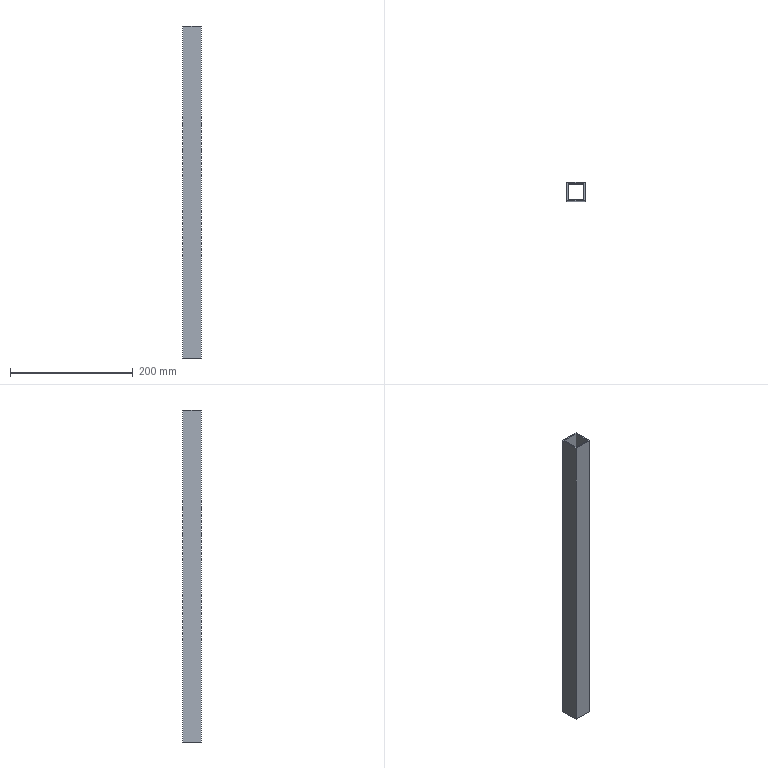Part | SolidWorks | features Extrusion 1 | 1 solid | 10 faces | box 30 x 30 x 540 mm | volume 120960 mm3 | plane 10
STEP:
#1=CARTESIAN_POINT('',(-15.,15.,270.));
#2=VERTEX_POINT('',#1);
#3=CARTESIAN_POINT('',(-15.,-15.,270.));
#4=VERTEX_POINT('',#3);
#5=CARTESIAN_POINT('',(-15.,-15.,270.));
#6=DIRECTION('',(0.,-1.,0.));
#7=VECTOR('',#6,1000.);
#8=LINE('',#5,#7);
#9=EDGE_CURVE('',#2,#4,#8,.T.);
#10=ORIENTED_EDGE('',*,*,#9,.T.);
#11=CARTESIAN_POINT('',(15.,-15.,270.));
#12=VERTEX_POINT('',#11);
#13=CARTESIAN_POINT('',(15.,-15.,270.));
#14=DIRECTION('',(1.,0.,0.));
#15=VECTOR('',#14,1000.);
#16=LINE('',#13,#15);
#17=EDGE_CURVE('',#4,#12,#16,.T.);
#18=ORIENTED_EDGE('',*,*,#17,.T.);
#19=CARTESIAN_POINT('',(15.,15.,270.));
#20=VERTEX_POINT('',#19);
#21=CARTESIAN_POINT('',(15.,-15.,270.));
#22=DIRECTION('',(0.,1.,0.));
#23=VECTOR('',#22,1000.);
#24=LINE('',#21,#23);
#25=EDGE_CURVE('',#12,#20,#24,.T.);
#26=ORIENTED_EDGE('',*,*,#25,.T.);
#27=CARTESIAN_POINT('',(15.,15.,270.));
#28=DIRECTION('',(-1.,0.,0.));
#29=VECTOR('',#28,1000.);
#30=LINE('',#27,#29);
#31=EDGE_CURVE('',#20,#2,#30,.T.);
#32=ORIENTED_EDGE('',*,*,#31,.T.);
#33=EDGE_LOOP('',(#10,#18,#26,#32));
#34=FACE_OUTER_BOUND('',#33,.T.);
#35=CARTESIAN_POINT('',(13.,13.,270.));
#36=VERTEX_POINT('',#35);
#37=CARTESIAN_POINT('',(-13.,13.,270.));
#38=VERTEX_POINT('',#37);
#39=CARTESIAN_POINT('',(13.,13.,270.));
#40=DIRECTION('',(-1.,0.,0.));
#41=VECTOR('',#40,1000.);
#42=LINE('',#39,#41);
#43=EDGE_CURVE('',#36,#38,#42,.T.);
#44=ORIENTED_EDGE('',*,*,#43,.F.);
#45=CARTESIAN_POINT('',(13.,-13.,270.));
#46=VERTEX_POINT('',#45);
#47=CARTESIAN_POINT('',(13.,-13.,270.));
#48=DIRECTION('',(0.,1.,0.));
#49=VECTOR('',#48,1000.);
#50=LINE('',#47,#49);
#51=EDGE_CURVE('',#46,#36,#50,.T.);
#52=ORIENTED_EDGE('',*,*,#51,.F.);
#53=CARTESIAN_POINT('',(-13.,-13.,270.));
#54=VERTEX_POINT('',#53);
#55=CARTESIAN_POINT('',(13.,-13.,270.));
#56=DIRECTION('',(1.,0.,0.));
#57=VECTOR('',#56,1000.);
#58=LINE('',#55,#57);
#59=EDGE_CURVE('',#54,#46,#58,.T.);
#60=ORIENTED_EDGE('',*,*,#59,.F.);
#61=CARTESIAN_POINT('',(-13.,-13.,270.));
#62=DIRECTION('',(0.,-1.,0.));
#63=VECTOR('',#62,1000.);
#64=LINE('',#61,#63);
#65=EDGE_CURVE('',#38,#54,#64,.T.);
#66=ORIENTED_EDGE('',*,*,#65,.F.);
#67=EDGE_LOOP('',(#44,#52,#60,#66));
#68=FACE_BOUND('',#67,.T.);
#69=CARTESIAN_POINT('',(0.,0.,270.));
#70=DIRECTION('',(0.,0.,1.));
#71=DIRECTION('',(1.,0.,0.));
#72=AXIS2_PLACEMENT_3D('',#69,#70,#71);
#73=PLANE('',#72);
#74=ADVANCED_FACE('',(#34,#68),#73,.T.);
#75=CARTESIAN_POINT('',(-15.,15.,-270.));
#76=VERTEX_POINT('',#75);
#77=CARTESIAN_POINT('',(-15.,-15.,-270.));
#78=VERTEX_POINT('',#77);
#79=CARTESIAN_POINT('',(-15.,-15.,-270.));
#80=DIRECTION('',(0.,-1.,0.));
#81=VECTOR('',#80,1000.);
#82=LINE('',#79,#81);
#83=EDGE_CURVE('',#76,#78,#82,.T.);
#84=ORIENTED_EDGE('',*,*,#83,.F.);
#85=CARTESIAN_POINT('',(15.,15.,-270.));
#86=VERTEX_POINT('',#85);
#87=CARTESIAN_POINT('',(15.,15.,-270.));
#88=DIRECTION('',(-1.,0.,0.));
#89=VECTOR('',#88,1000.);
#90=LINE('',#87,#89);
#91=EDGE_CURVE('',#86,#76,#90,.T.);
#92=ORIENTED_EDGE('',*,*,#91,.F.);
#93=CARTESIAN_POINT('',(15.,-15.,-270.));
#94=VERTEX_POINT('',#93);
#95=CARTESIAN_POINT('',(15.,-15.,-270.));
#96=DIRECTION('',(0.,1.,0.));
#97=VECTOR('',#96,1000.);
#98=LINE('',#95,#97);
#99=EDGE_CURVE('',#94,#86,#98,.T.);
#100=ORIENTED_EDGE('',*,*,#99,.F.);
#101=CARTESIAN_POINT('',(15.,-15.,-270.));
#102=DIRECTION('',(1.,0.,0.));
#103=VECTOR('',#102,1000.);
#104=LINE('',#101,#103);
#105=EDGE_CURVE('',#78,#94,#104,.T.);
#106=ORIENTED_EDGE('',*,*,#105,.F.);
#107=EDGE_LOOP('',(#84,#92,#100,#106));
#108=FACE_OUTER_BOUND('',#107,.T.);
#109=CARTESIAN_POINT('',(13.,-13.,-270.));
#110=VERTEX_POINT('',#109);
#111=CARTESIAN_POINT('',(13.,13.,-270.));
#112=VERTEX_POINT('',#111);
#113=CARTESIAN_POINT('',(13.,-13.,-270.));
#114=DIRECTION('',(0.,1.,0.));
#115=VECTOR('',#114,1000.);
#116=LINE('',#113,#115);
#117=EDGE_CURVE('',#110,#112,#116,.T.);
#118=ORIENTED_EDGE('',*,*,#117,.T.);
#119=CARTESIAN_POINT('',(-13.,13.,-270.));
#120=VERTEX_POINT('',#119);
#121=CARTESIAN_POINT('',(13.,13.,-270.));
#122=DIRECTION('',(-1.,0.,0.));
#123=VECTOR('',#122,1000.);
#124=LINE('',#121,#123);
#125=EDGE_CURVE('',#112,#120,#124,.T.);
#126=ORIENTED_EDGE('',*,*,#125,.T.);
#127=CARTESIAN_POINT('',(-13.,-13.,-270.));
#128=VERTEX_POINT('',#127);
#129=CARTESIAN_POINT('',(-13.,-13.,-270.));
#130=DIRECTION('',(0.,-1.,0.));
#131=VECTOR('',#130,1000.);
#132=LINE('',#129,#131);
#133=EDGE_CURVE('',#120,#128,#132,.T.);
#134=ORIENTED_EDGE('',*,*,#133,.T.);
#135=CARTESIAN_POINT('',(13.,-13.,-270.));
#136=DIRECTION('',(1.,0.,0.));
#137=VECTOR('',#136,1000.);
#138=LINE('',#135,#137);
#139=EDGE_CURVE('',#128,#110,#138,.T.);
#140=ORIENTED_EDGE('',*,*,#139,.T.);
#141=EDGE_LOOP('',(#118,#126,#134,#140));
#142=FACE_BOUND('',#141,.T.);
#143=CARTESIAN_POINT('',(0.,0.,-270.));
#144=DIRECTION('',(0.,0.,1.));
#145=DIRECTION('',(1.,0.,0.));
#146=AXIS2_PLACEMENT_3D('',#143,#144,#145);
#147=PLANE('',#146);
#148=ADVANCED_FACE('',(#108,#142),#147,.F.);
#149=ORIENTED_EDGE('',*,*,#83,.T.);
#150=CARTESIAN_POINT('',(-15.,-15.,270.));
#151=DIRECTION('',(0.,0.,-1.));
#152=VECTOR('',#151,1000.);
#153=LINE('',#150,#152);
#154=EDGE_CURVE('',#4,#78,#153,.T.);
#155=ORIENTED_EDGE('',*,*,#154,.F.);
#156=ORIENTED_EDGE('',*,*,#9,.F.);
#157=CARTESIAN_POINT('',(-15.,15.,270.));
#158=DIRECTION('',(0.,0.,-1.));
#159=VECTOR('',#158,1000.);
#160=LINE('',#157,#159);
#161=EDGE_CURVE('',#2,#76,#160,.T.);
#162=ORIENTED_EDGE('',*,*,#161,.T.);
#163=EDGE_LOOP('',(#149,#155,#156,#162));
#164=FACE_OUTER_BOUND('',#163,.T.);
#165=CARTESIAN_POINT('',(-15.,-15.,270.));
#166=DIRECTION('',(1.,0.,0.));
#167=DIRECTION('',(0.,1.,0.));
#168=AXIS2_PLACEMENT_3D('',#165,#166,#167);
#169=PLANE('',#168);
#170=ADVANCED_FACE('',(#164),#169,.F.);
#171=ORIENTED_EDGE('',*,*,#105,.T.);
#172=CARTESIAN_POINT('',(15.,-15.,270.));
#173=DIRECTION('',(0.,0.,-1.));
#174=VECTOR('',#173,1000.);
#175=LINE('',#172,#174);
#176=EDGE_CURVE('',#12,#94,#175,.T.);
#177=ORIENTED_EDGE('',*,*,#176,.F.);
#178=ORIENTED_EDGE('',*,*,#17,.F.);
#179=ORIENTED_EDGE('',*,*,#154,.T.);
#180=EDGE_LOOP('',(#171,#177,#178,#179));
#181=FACE_OUTER_BOUND('',#180,.T.);
#182=CARTESIAN_POINT('',(15.,-15.,270.));
#183=DIRECTION('',(0.,1.,0.));
#184=DIRECTION('',(-1.,0.,0.));
#185=AXIS2_PLACEMENT_3D('',#182,#183,#184);
#186=PLANE('',#185);
#187=ADVANCED_FACE('',(#181),#186,.F.);
#188=ORIENTED_EDGE('',*,*,#99,.T.);
#189=CARTESIAN_POINT('',(15.,15.,270.));
#190=DIRECTION('',(0.,0.,-1.));
#191=VECTOR('',#190,1000.);
#192=LINE('',#189,#191);
#193=EDGE_CURVE('',#20,#86,#192,.T.);
#194=ORIENTED_EDGE('',*,*,#193,.F.);
#195=ORIENTED_EDGE('',*,*,#25,.F.);
#196=ORIENTED_EDGE('',*,*,#176,.T.);
#197=EDGE_LOOP('',(#188,#194,#195,#196));
#198=FACE_OUTER_BOUND('',#197,.T.);
#199=CARTESIAN_POINT('',(15.,-15.,270.));
#200=DIRECTION('',(-1.,0.,0.));
#201=DIRECTION('',(0.,0.,1.));
#202=AXIS2_PLACEMENT_3D('',#199,#200,#201);
#203=PLANE('',#202);
#204=ADVANCED_FACE('',(#198),#203,.F.);
#205=ORIENTED_EDGE('',*,*,#91,.T.);
#206=ORIENTED_EDGE('',*,*,#161,.F.);
#207=ORIENTED_EDGE('',*,*,#31,.F.);
#208=ORIENTED_EDGE('',*,*,#193,.T.);
#209=EDGE_LOOP('',(#205,#206,#207,#208));
#210=FACE_OUTER_BOUND('',#209,.T.);
#211=CARTESIAN_POINT('',(15.,15.,270.));
#212=DIRECTION('',(0.,-1.,0.));
#213=DIRECTION('',(0.,0.,-1.));
#214=AXIS2_PLACEMENT_3D('',#211,#212,#213);
#215=PLANE('',#214);
#216=ADVANCED_FACE('',(#210),#215,.F.);
#217=ORIENTED_EDGE('',*,*,#117,.F.);
#218=CARTESIAN_POINT('',(13.,-13.,270.));
#219=DIRECTION('',(0.,0.,-1.));
#220=VECTOR('',#219,1000.);
#221=LINE('',#218,#220);
#222=EDGE_CURVE('',#46,#110,#221,.T.);
#223=ORIENTED_EDGE('',*,*,#222,.F.);
#224=ORIENTED_EDGE('',*,*,#51,.T.);
#225=CARTESIAN_POINT('',(13.,13.,270.));
#226=DIRECTION('',(0.,0.,-1.));
#227=VECTOR('',#226,1000.);
#228=LINE('',#225,#227);
#229=EDGE_CURVE('',#36,#112,#228,.T.);
#230=ORIENTED_EDGE('',*,*,#229,.T.);
#231=EDGE_LOOP('',(#217,#223,#224,#230));
#232=FACE_OUTER_BOUND('',#231,.T.);
#233=CARTESIAN_POINT('',(13.,-13.,270.));
#234=DIRECTION('',(-1.,0.,0.));
#235=DIRECTION('',(0.,0.,1.));
#236=AXIS2_PLACEMENT_3D('',#233,#234,#235);
#237=PLANE('',#236);
#238=ADVANCED_FACE('',(#232),#237,.T.);
#239=ORIENTED_EDGE('',*,*,#125,.F.);
#240=ORIENTED_EDGE('',*,*,#229,.F.);
#241=ORIENTED_EDGE('',*,*,#43,.T.);
#242=CARTESIAN_POINT('',(-13.,13.,270.));
#243=DIRECTION('',(0.,0.,-1.));
#244=VECTOR('',#243,1000.);
#245=LINE('',#242,#244);
#246=EDGE_CURVE('',#38,#120,#245,.T.);
#247=ORIENTED_EDGE('',*,*,#246,.T.);
#248=EDGE_LOOP('',(#239,#240,#241,#247));
#249=FACE_OUTER_BOUND('',#248,.T.);
#250=CARTESIAN_POINT('',(13.,13.,270.));
#251=DIRECTION('',(0.,-1.,0.));
#252=DIRECTION('',(0.,0.,-1.));
#253=AXIS2_PLACEMENT_3D('',#250,#251,#252);
#254=PLANE('',#253);
#255=ADVANCED_FACE('',(#249),#254,.T.);
#256=ORIENTED_EDGE('',*,*,#133,.F.);
#257=ORIENTED_EDGE('',*,*,#246,.F.);
#258=ORIENTED_EDGE('',*,*,#65,.T.);
#259=CARTESIAN_POINT('',(-13.,-13.,270.));
#260=DIRECTION('',(0.,0.,-1.));
#261=VECTOR('',#260,1000.);
#262=LINE('',#259,#261);
#263=EDGE_CURVE('',#54,#128,#262,.T.);
#264=ORIENTED_EDGE('',*,*,#263,.T.);
#265=EDGE_LOOP('',(#256,#257,#258,#264));
#266=FACE_OUTER_BOUND('',#265,.T.);
#267=CARTESIAN_POINT('',(-13.,-13.,270.));
#268=DIRECTION('',(1.,0.,0.));
#269=DIRECTION('',(0.,0.,-1.));
#270=AXIS2_PLACEMENT_3D('',#267,#268,#269);
#271=PLANE('',#270);
#272=ADVANCED_FACE('',(#266),#271,.T.);
#273=ORIENTED_EDGE('',*,*,#139,.F.);
#274=ORIENTED_EDGE('',*,*,#263,.F.);
#275=ORIENTED_EDGE('',*,*,#59,.T.);
#276=ORIENTED_EDGE('',*,*,#222,.T.);
#277=EDGE_LOOP('',(#273,#274,#275,#276));
#278=FACE_OUTER_BOUND('',#277,.T.);
#279=CARTESIAN_POINT('',(13.,-13.,270.));
#280=DIRECTION('',(0.,1.,0.));
#281=DIRECTION('',(0.,0.,1.));
#282=AXIS2_PLACEMENT_3D('',#279,#280,#281);
#283=PLANE('',#282);
#284=ADVANCED_FACE('',(#278),#283,.T.);
#285=CLOSED_SHELL('',(#74,#148,#170,#187,#204,#216,#238,#255,#272,#284));
#286=MANIFOLD_SOLID_BREP('',#285);
#287=CARTESIAN_POINT('',(0.,0.,0.));
#288=DIRECTION('',(0.,0.,1.));
#289=DIRECTION('',(1.,0.,0.));
#290=AXIS2_PLACEMENT_3D('',#287,#288,#289);
#291=(LENGTH_UNIT()NAMED_UNIT(*)SI_UNIT(.MILLI.,.METRE.));
#292=UNCERTAINTY_MEASURE_WITH_UNIT(LENGTH_MEASURE(0.00001),#291,'','');
#293=(NAMED_UNIT(*)PLANE_ANGLE_UNIT()SI_UNIT($,.RADIAN.));
#294=(NAMED_UNIT(*)SI_UNIT($,.STERADIAN.)SOLID_ANGLE_UNIT());
#295=(GEOMETRIC_REPRESENTATION_CONTEXT(3)GLOBAL_UNCERTAINTY_ASSIGNED_CONTEXT((#292))GLOBAL_UNIT_ASSIGNED_CONTEXT((#291,#293,#294))REPRESENTATION_CONTEXT('',''));
#296=ADVANCED_BREP_SHAPE_REPRESENTATION('',(#286,#290),#295);